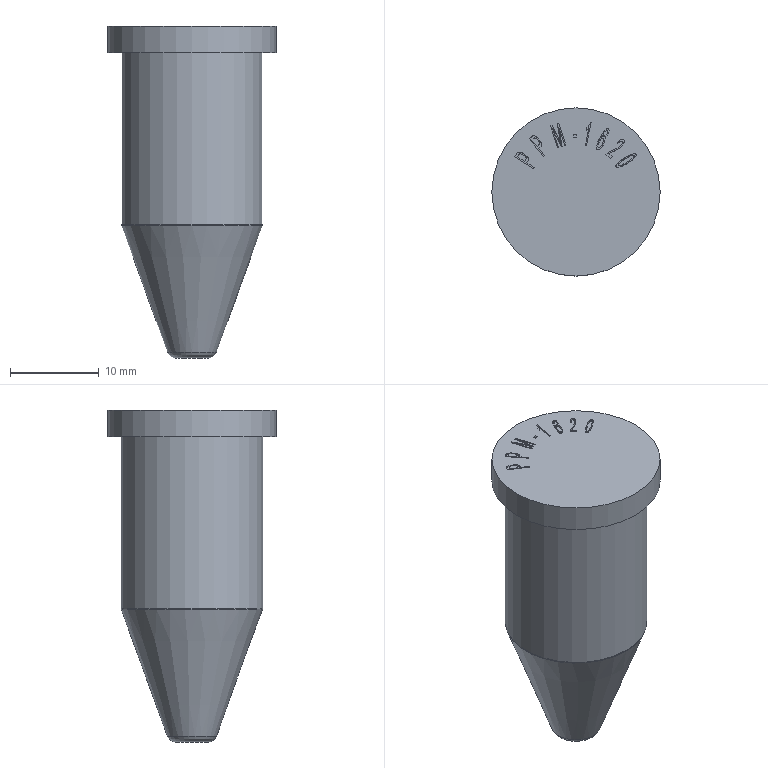Part | STEP file | lll_id2798_x_t | 1 solid | 77 faces | box 19 x 19 x 37.5 mm | volume 6195 mm3 | plane 48 | other 24 | cylinder 2 | torus 2 | cone 1 | commonest cylinder face diameters 16 x1 19 x1